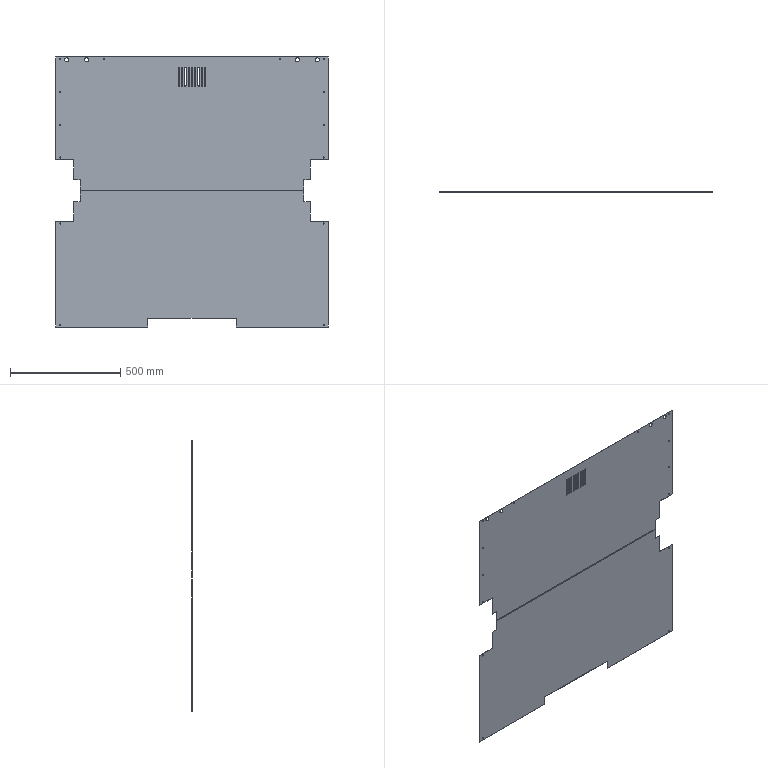Part | 2 solids | 104 faces | box 1240 x 1 x 1226 mm | volume 1445041 mm3 | cylinder 54 | plane 50 | commonest cylinder face diameters 5 x28 6 x18 18 x8